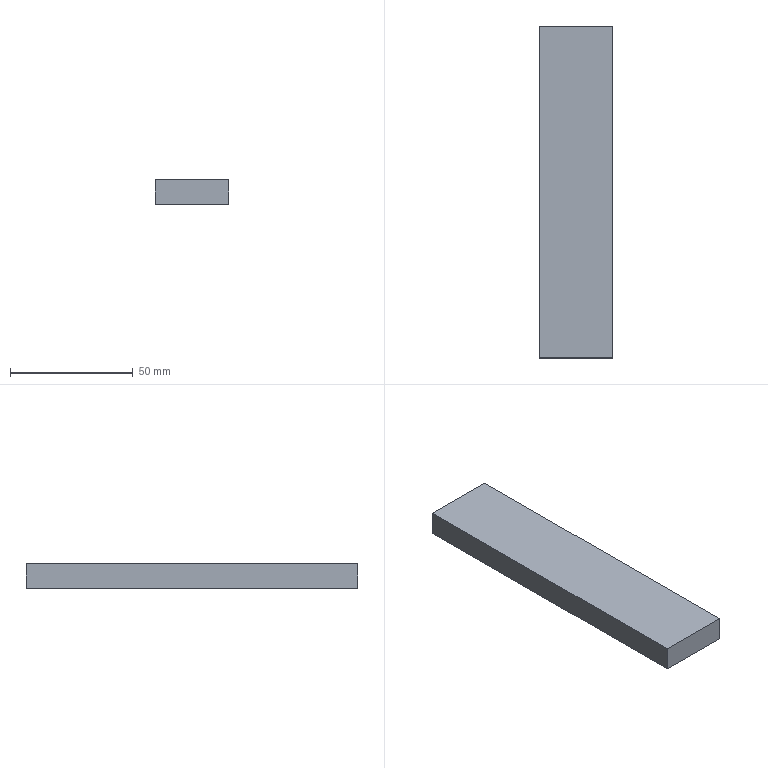Part | NX | features solid 2 | 1 solid | 6 faces | box 30 x 135 x 10 mm | volume 40500 mm3 | plane 6
STEP:
#1=CARTESIAN_POINT('',(-565.,110.,-55.));
#2=VERTEX_POINT('',#1);
#3=CARTESIAN_POINT('',(-565.,110.,-65.));
#4=VERTEX_POINT('',#3);
#5=CARTESIAN_POINT('',(-565.,110.,-65.));
#6=DIRECTION('',(0.,0.,-1.));
#7=VECTOR('',#6,1000.);
#8=LINE('',#5,#7);
#9=EDGE_CURVE('',#2,#4,#8,.T.);
#10=ORIENTED_EDGE('',*,*,#9,.T.);
#11=CARTESIAN_POINT('',(-595.,110.,-65.));
#12=VERTEX_POINT('',#11);
#13=CARTESIAN_POINT('',(-610.,110.,-65.));
#14=DIRECTION('',(-1.,0.,0.));
#15=VECTOR('',#14,1000.);
#16=LINE('',#13,#15);
#17=EDGE_CURVE('',#12,#4,#16,.F.);
#18=ORIENTED_EDGE('',*,*,#17,.F.);
#19=CARTESIAN_POINT('',(-595.,110.,-55.));
#20=VERTEX_POINT('',#19);
#21=CARTESIAN_POINT('',(-595.,110.,-65.));
#22=DIRECTION('',(0.,0.,-1.));
#23=VECTOR('',#22,1000.);
#24=LINE('',#21,#23);
#25=EDGE_CURVE('',#20,#12,#24,.T.);
#26=ORIENTED_EDGE('',*,*,#25,.F.);
#27=CARTESIAN_POINT('',(-610.,110.,-55.));
#28=DIRECTION('',(-1.,0.,0.));
#29=VECTOR('',#28,1000.);
#30=LINE('',#27,#29);
#31=EDGE_CURVE('',#2,#20,#30,.T.);
#32=ORIENTED_EDGE('',*,*,#31,.F.);
#33=EDGE_LOOP('',(#10,#18,#26,#32));
#34=FACE_BOUND('',#33,.T.);
#35=CARTESIAN_POINT('',(-540.,110.,-55.));
#36=DIRECTION('',(0.,-1.,0.));
#37=DIRECTION('',(0.,0.,-1.));
#38=AXIS2_PLACEMENT_3D('',#35,#36,#37);
#39=PLANE('',#38);
#40=ADVANCED_FACE('',(#34),#39,.F.);
#41=CARTESIAN_POINT('',(-595.,-25.,-65.));
#42=VERTEX_POINT('',#41);
#43=CARTESIAN_POINT('',(-595.,110.,-65.));
#44=DIRECTION('',(0.,1.,0.));
#45=VECTOR('',#44,1000.);
#46=LINE('',#43,#45);
#47=EDGE_CURVE('',#42,#12,#46,.T.);
#48=ORIENTED_EDGE('',*,*,#47,.F.);
#49=CARTESIAN_POINT('',(-595.,-25.,-55.));
#50=VERTEX_POINT('',#49);
#51=CARTESIAN_POINT('',(-595.,-25.,-65.));
#52=DIRECTION('',(0.,0.,1.));
#53=VECTOR('',#52,1000.);
#54=LINE('',#51,#53);
#55=EDGE_CURVE('',#42,#50,#54,.T.);
#56=ORIENTED_EDGE('',*,*,#55,.T.);
#57=CARTESIAN_POINT('',(-595.,110.,-55.));
#58=DIRECTION('',(0.,1.,0.));
#59=VECTOR('',#58,1000.);
#60=LINE('',#57,#59);
#61=EDGE_CURVE('',#50,#20,#60,.T.);
#62=ORIENTED_EDGE('',*,*,#61,.T.);
#63=ORIENTED_EDGE('',*,*,#25,.T.);
#64=EDGE_LOOP('',(#48,#56,#62,#63));
#65=FACE_BOUND('',#64,.T.);
#66=CARTESIAN_POINT('',(-595.,110.,-65.));
#67=DIRECTION('',(1.,0.,0.));
#68=DIRECTION('',(0.,0.,-1.));
#69=AXIS2_PLACEMENT_3D('',#66,#67,#68);
#70=PLANE('',#69);
#71=ADVANCED_FACE('',(#65),#70,.F.);
#72=ORIENTED_EDGE('',*,*,#9,.F.);
#73=CARTESIAN_POINT('',(-565.,-25.,-55.));
#74=VERTEX_POINT('',#73);
#75=CARTESIAN_POINT('',(-565.,110.,-55.));
#76=DIRECTION('',(0.,1.,0.));
#77=VECTOR('',#76,1000.);
#78=LINE('',#75,#77);
#79=EDGE_CURVE('',#74,#2,#78,.T.);
#80=ORIENTED_EDGE('',*,*,#79,.F.);
#81=CARTESIAN_POINT('',(-565.,-25.,-65.));
#82=VERTEX_POINT('',#81);
#83=CARTESIAN_POINT('',(-565.,-25.,-65.));
#84=DIRECTION('',(0.,0.,-1.));
#85=VECTOR('',#84,1000.);
#86=LINE('',#83,#85);
#87=EDGE_CURVE('',#74,#82,#86,.T.);
#88=ORIENTED_EDGE('',*,*,#87,.T.);
#89=CARTESIAN_POINT('',(-565.,110.,-65.));
#90=DIRECTION('',(0.,1.,0.));
#91=VECTOR('',#90,1000.);
#92=LINE('',#89,#91);
#93=EDGE_CURVE('',#82,#4,#92,.T.);
#94=ORIENTED_EDGE('',*,*,#93,.T.);
#95=EDGE_LOOP('',(#72,#80,#88,#94));
#96=FACE_BOUND('',#95,.T.);
#97=CARTESIAN_POINT('',(-565.,110.,-65.));
#98=DIRECTION('',(1.,0.,0.));
#99=DIRECTION('',(0.,0.,-1.));
#100=AXIS2_PLACEMENT_3D('',#97,#98,#99);
#101=PLANE('',#100);
#102=ADVANCED_FACE('',(#96),#101,.T.);
#103=ORIENTED_EDGE('',*,*,#93,.F.);
#104=CARTESIAN_POINT('',(-610.,-25.,-65.));
#105=DIRECTION('',(1.,0.,0.));
#106=VECTOR('',#105,1000.);
#107=LINE('',#104,#106);
#108=EDGE_CURVE('',#82,#42,#107,.F.);
#109=ORIENTED_EDGE('',*,*,#108,.T.);
#110=ORIENTED_EDGE('',*,*,#47,.T.);
#111=ORIENTED_EDGE('',*,*,#17,.T.);
#112=EDGE_LOOP('',(#103,#109,#110,#111));
#113=FACE_BOUND('',#112,.T.);
#114=CARTESIAN_POINT('',(-610.,110.,-65.));
#115=DIRECTION('',(0.,0.,-1.));
#116=DIRECTION('',(0.,1.,0.));
#117=AXIS2_PLACEMENT_3D('',#114,#115,#116);
#118=PLANE('',#117);
#119=ADVANCED_FACE('',(#113),#118,.T.);
#120=ORIENTED_EDGE('',*,*,#61,.F.);
#121=CARTESIAN_POINT('',(-610.,-25.,-55.));
#122=DIRECTION('',(1.,0.,0.));
#123=VECTOR('',#122,1000.);
#124=LINE('',#121,#123);
#125=EDGE_CURVE('',#50,#74,#124,.T.);
#126=ORIENTED_EDGE('',*,*,#125,.T.);
#127=ORIENTED_EDGE('',*,*,#79,.T.);
#128=ORIENTED_EDGE('',*,*,#31,.T.);
#129=EDGE_LOOP('',(#120,#126,#127,#128));
#130=FACE_BOUND('',#129,.T.);
#131=CARTESIAN_POINT('',(-610.,110.,-55.));
#132=DIRECTION('',(0.,0.,-1.));
#133=DIRECTION('',(0.,1.,0.));
#134=AXIS2_PLACEMENT_3D('',#131,#132,#133);
#135=PLANE('',#134);
#136=ADVANCED_FACE('',(#130),#135,.F.);
#137=ORIENTED_EDGE('',*,*,#55,.F.);
#138=ORIENTED_EDGE('',*,*,#108,.F.);
#139=ORIENTED_EDGE('',*,*,#87,.F.);
#140=ORIENTED_EDGE('',*,*,#125,.F.);
#141=EDGE_LOOP('',(#137,#138,#139,#140));
#142=FACE_BOUND('',#141,.T.);
#143=CARTESIAN_POINT('',(-525.,-25.,0.));
#144=DIRECTION('',(0.,1.,0.));
#145=DIRECTION('',(0.,0.,1.));
#146=AXIS2_PLACEMENT_3D('',#143,#144,#145);
#147=PLANE('',#146);
#148=ADVANCED_FACE('',(#142),#147,.F.);
#149=CLOSED_SHELL('',(#40,#71,#102,#119,#136,#148));
#150=MANIFOLD_SOLID_BREP('',#149);
#151=(LENGTH_UNIT()NAMED_UNIT(*)SI_UNIT(.MILLI.,.METRE.));
#152=UNCERTAINTY_MEASURE_WITH_UNIT(LENGTH_MEASURE(0.00001),#151,'','');
#153=(NAMED_UNIT(*)PLANE_ANGLE_UNIT()SI_UNIT($,.RADIAN.));
#154=(NAMED_UNIT(*)SI_UNIT($,.STERADIAN.)SOLID_ANGLE_UNIT());
#155=(GEOMETRIC_REPRESENTATION_CONTEXT(3)GLOBAL_UNCERTAINTY_ASSIGNED_CONTEXT((#152))GLOBAL_UNIT_ASSIGNED_CONTEXT((#151,#153,#154))REPRESENTATION_CONTEXT('',''));
#156=ADVANCED_BREP_SHAPE_REPRESENTATION('',(#150),#155);